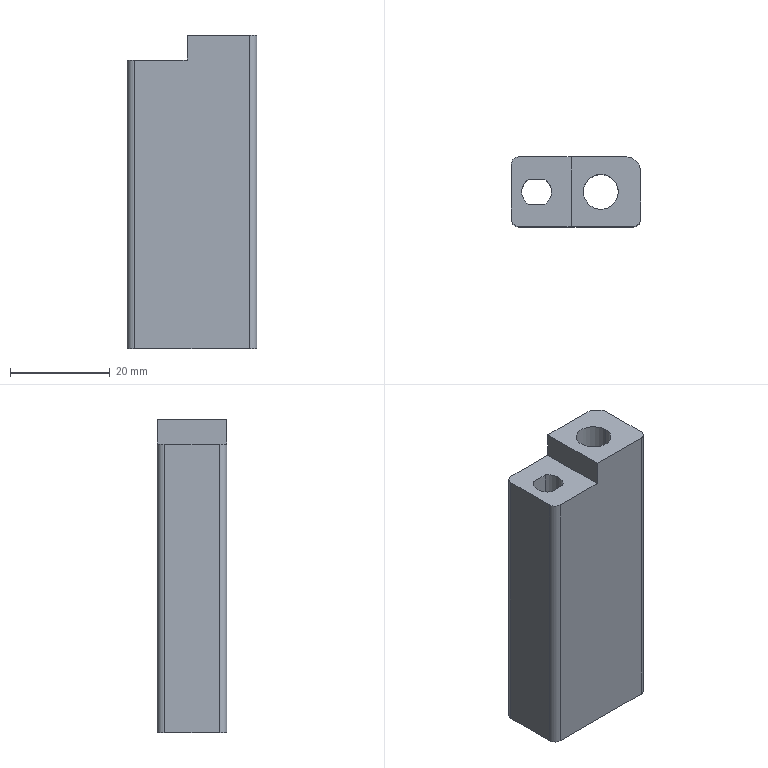Part | 1 solid | 21 faces | box 26 x 14 x 63 mm | volume 17385 mm3 | plane 11 | cylinder 10 | commonest cylinder face diameters 3 x3 6 x3 7 x2 11 x2